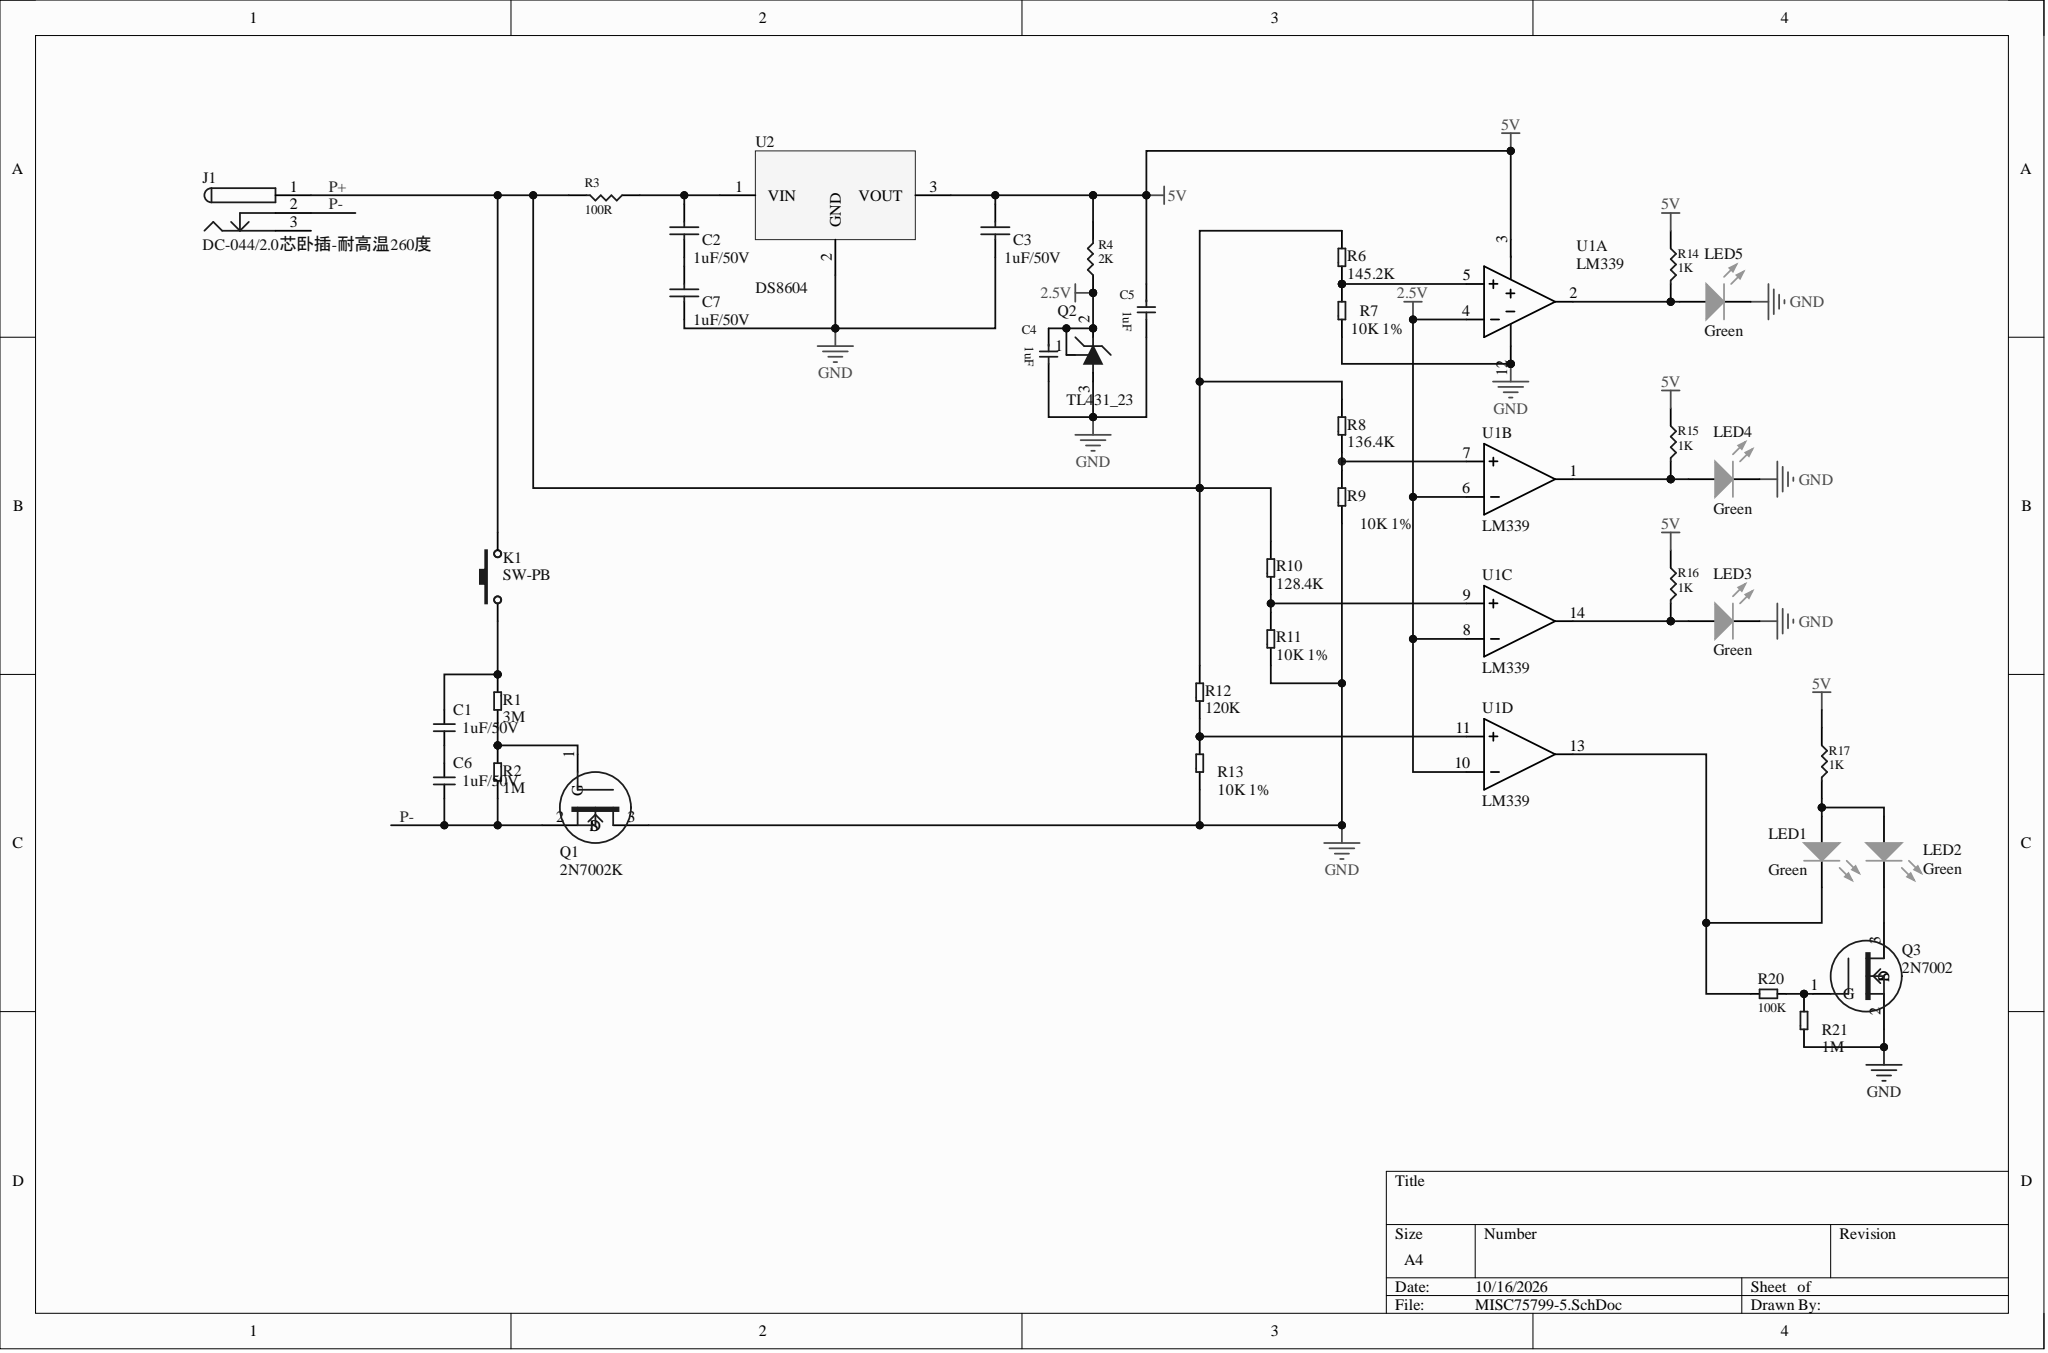Circuit board | Altium Designer | 37 parts | 21 nets
Bill of materials:
Comment,Description,Designator,Footprint,LibRef,Quantity
"1uF/50V","0603 SMD capacitor, Capacitor","C1, C2, C3, C6, C7","C0603A","C0603, Cap","5"
"1uF","","C4, C5","C0603A","0.1u","2"
"DC-044/2.0芯卧插-耐高温260度","DC-044 power connector - Yueqing Jinghong","J1","DC-044","DC-044/2.0芯卧插-耐高温260度","1"
"SW-PB","6*6 tactile switch","K1","SW-SMD_4P-L12.0-W12.0-P5.00-LS15.2","SW-PB_1","1"
"Green","SMD LED lamp","LED1, LED2, LED3, LED4, LED5","LED0603A","LED_Green","5"
"2N7002K","","Q1","SOT23-3","NMOS","1"
"TL431_23","IC SOT-23","Q2","SOT23-3","TL431_23","1"
"2N7002","","Q3","SOT23-3","NMOS","1"
"3M","","R1","R0603A","R","1"
"1M","","R2, R21","R0603A","R","2"
"100R","","R3","R0805A","RES","1"
"2K","","R4","R0805A","RES","1"
"145.2K","","R6","R0603A","R","1"
"10K 1%","","R7, R9, R11, R13","R0603A","R","4"
"136.4K","","R8","R0603A","R","1"
"128.4K","","R10","R0603A","R","1"
"120K","","R12","R0603A","R","1"
"1K","","R14, R15, R16, R17","R0603A","RES","4"
"100K","","R20","R0603A","R-S","1"
"LM339","LM339","U1","SOP14L","LM339","1"
"DS8604","LDO","U2","SOT-89-3","LDO DS8604","1"
Netlist (Protel format):
[
C1
C0603A
1uF/50V



]
[
C2
C0603A
1uF/50V



]
[
C3
C0603A
1uF/50V



]
[
C4
C0603A
1uF



]
[
C5
C0603A
1uF



]
[
C6
C0603A
1uF/50V



]
[
C7
C0603A
1uF/50V



]
[
J1
DC-044
DC-044/2.0芯卧插-耐高温260度



]
[
K1
SW-SMD_4P-L12.0-W12.0-P5.00-LS15.2
SW-PB



]
[
LED1
LED0603A
Green



]
[
LED2
LED0603A
Green



]
[
LED3
LED0603A
Green



]
[
LED4
LED0603A
Green



]
[
LED5
LED0603A
Green



]
[
Q1
SOT23-3
2N7002K



]
[
Q2
SOT23-3
TL431_23



]
[
Q3
SOT23-3
2N7002



]
[
R1
R0603A
3M



]
[
R2
R0603A
1M



]
[
R3
R0805A
100R



]
[
R4
R0805A
2K



]
[
R6
R0603A
145.2K



]
[
R7
R0603A
10K 1%



]
[
R8
R0603A
136.4K



]
[
R9
R0603A
10K 1%



]
[
R10
R0603A
128.4K



]
[
R11
R0603A
10K 1%



]
[
R12
R0603A
120K



]
[
R13
R0603A
10K 1%



]
[
R14
R0603A
1K



]
[
R15
R0603A
1K



]
[
R16
R0603A
1K



]
[
R17
R0603A
1K



]
[
R20
R0603A
100K



]
[
R21
R0603A
1M



]
[
U1
SOP14L
LM339



]
[
U2
SOT-89-3
DS8604



]
(
P-
C6-2
J1-2
Q1-2
R2-2
)
(
P+
J1-1
K1-2
R3-2
R6-2
R8-2
R10-2
R12-2
)
(
NetR12_1
R12-1
R13-2
U1-11
)
(
NetR10_1
R10-1
R11-2
U1-9
)
(
NetR8_1
R8-1
R9-2
U1-7
)
(
NetR6_1
R6-1
R7-2
U1-5
)
(
NetQ3_1
Q3-1
R20-1
R21-2
)
(
NetQ1_1
Q1-1
R1-2
R2-1
)
(
NetLED5_2
LED5-2
R14-2
U1-2
)
(
NetLED4_2
LED4-2
R15-2
U1-1
)
(
NetLED3_2
LED3-2
R16-2
U1-14
)
(
NetLED2_1
LED2-1
Q3-3
)
(
NetLED1_2
LED1-2
LED2-2
R17-2
)
(
NetLED1_1
LED1-1
R20-2
U1-13
)
(
NetC2_2
C2-2
R3-1
U2-1
)
(
NetC2_1
C2-1
C7-2
)
(
NetC1_2
C1-2
C6-1
)
(
NetC1_1
C1-1
K1-1
R1-1
)
(
GND
C3-1
C4-1
C5-1
C7-1
LED3-1
LED4-1
LED5-1
Q1-3
Q2-3
Q3-2
R7-1
R9-1
R11-1
R13-1
R21-1
U1-12
U2-2
)
(
5V
C3-2
C5-2
R4-2
R14-1
R15-1
R16-1
R17-1
U1-3
U2-3
)
(
2.5V
C4-2
Q2-1
Q2-2
R4-1
U1-4
U1-6
U1-8
U1-10
)